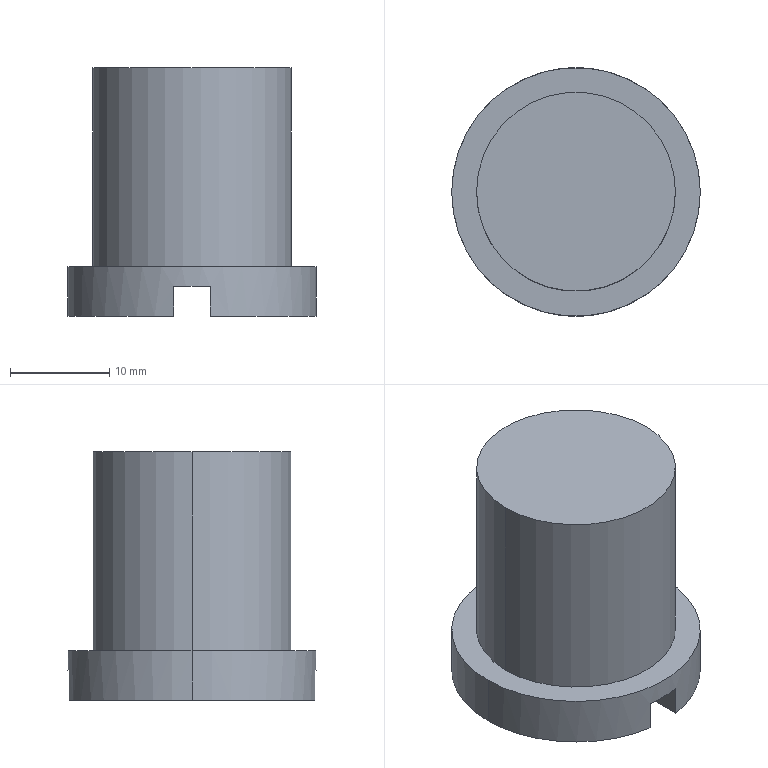Part | SolidWorks | features ICE 2, Extrusion 1 | 1 solid | 11 faces | box 25 x 25 x 25 mm | volume 8464 mm3 | plane 7 | cylinder 4 | commonest cylinder face diameters 20 x2 25 x2
STEP:
#1=CARTESIAN_POINT('',(10.,0.,25.));
#2=VERTEX_POINT('',#1);
#3=CARTESIAN_POINT('',(-10.,0.,25.));
#4=VERTEX_POINT('',#3);
#5=CARTESIAN_POINT('',(0.,0.,25.));
#6=DIRECTION('',(0.,0.,1.));
#7=DIRECTION('',(1.,0.,0.));
#8=AXIS2_PLACEMENT_3D('',#5,#6,#7);
#9=CIRCLE('',#8,10.);
#10=EDGE_CURVE('',#2,#4,#9,.T.);
#11=ORIENTED_EDGE('',*,*,#10,.F.);
#12=CARTESIAN_POINT('',(10.,0.,5.));
#13=VERTEX_POINT('',#12);
#14=CARTESIAN_POINT('',(10.,0.,25.));
#15=DIRECTION('',(0.,0.,-1.));
#16=VECTOR('',#15,1000.);
#17=LINE('',#14,#16);
#18=EDGE_CURVE('',#2,#13,#17,.T.);
#19=ORIENTED_EDGE('',*,*,#18,.T.);
#20=CARTESIAN_POINT('',(-10.,0.,5.));
#21=VERTEX_POINT('',#20);
#22=CARTESIAN_POINT('',(0.,0.,5.));
#23=DIRECTION('',(0.,0.,1.));
#24=DIRECTION('',(1.,0.,0.));
#25=AXIS2_PLACEMENT_3D('',#22,#23,#24);
#26=CIRCLE('',#25,10.);
#27=EDGE_CURVE('',#13,#21,#26,.T.);
#28=ORIENTED_EDGE('',*,*,#27,.T.);
#29=CARTESIAN_POINT('',(-10.,0.,25.));
#30=DIRECTION('',(0.,0.,-1.));
#31=VECTOR('',#30,1000.);
#32=LINE('',#29,#31);
#33=EDGE_CURVE('',#4,#21,#32,.T.);
#34=ORIENTED_EDGE('',*,*,#33,.F.);
#35=EDGE_LOOP('',(#11,#19,#28,#34));
#36=FACE_OUTER_BOUND('',#35,.T.);
#37=CARTESIAN_POINT('',(0.,0.,25.));
#38=DIRECTION('',(0.,0.,-1.));
#39=DIRECTION('',(-1.,0.,0.));
#40=AXIS2_PLACEMENT_3D('',#37,#38,#39);
#41=CYLINDRICAL_SURFACE('',#40,10.);
#42=ADVANCED_FACE('',(#36),#41,.T.);
#43=CARTESIAN_POINT('',(12.5,0.,5.));
#44=VERTEX_POINT('',#43);
#45=CARTESIAN_POINT('',(-12.5,0.,5.));
#46=VERTEX_POINT('',#45);
#47=CARTESIAN_POINT('',(0.,0.,5.));
#48=DIRECTION('',(0.,0.,1.));
#49=DIRECTION('',(1.,0.,0.));
#50=AXIS2_PLACEMENT_3D('',#47,#48,#49);
#51=CIRCLE('',#50,12.5);
#52=EDGE_CURVE('',#44,#46,#51,.T.);
#53=ORIENTED_EDGE('',*,*,#52,.F.);
#54=CARTESIAN_POINT('',(12.5,0.,0.));
#55=VERTEX_POINT('',#54);
#56=CARTESIAN_POINT('',(12.5,0.,5.));
#57=DIRECTION('',(0.,0.,-1.));
#58=VECTOR('',#57,1000.);
#59=LINE('',#56,#58);
#60=EDGE_CURVE('',#44,#55,#59,.T.);
#61=ORIENTED_EDGE('',*,*,#60,.T.);
#62=CARTESIAN_POINT('',(1.832,12.365,0.));
#63=VERTEX_POINT('',#62);
#64=CARTESIAN_POINT('',(0.,0.,0.));
#65=DIRECTION('',(0.,0.,1.));
#66=DIRECTION('',(1.,0.,0.));
#67=AXIS2_PLACEMENT_3D('',#64,#65,#66);
#68=CIRCLE('',#67,12.5);
#69=EDGE_CURVE('',#55,#63,#68,.T.);
#70=ORIENTED_EDGE('',*,*,#69,.T.);
#71=CARTESIAN_POINT('',(1.832,12.365,3.));
#72=VERTEX_POINT('',#71);
#73=CARTESIAN_POINT('',(1.832,12.365,3.));
#74=DIRECTION('',(0.,0.,-1.));
#75=VECTOR('',#74,1000.);
#76=LINE('',#73,#75);
#77=EDGE_CURVE('',#72,#63,#76,.T.);
#78=ORIENTED_EDGE('',*,*,#77,.F.);
#79=CARTESIAN_POINT('',(-1.832,12.365,3.));
#80=VERTEX_POINT('',#79);
#81=CARTESIAN_POINT('',(0.,0.,3.));
#82=DIRECTION('',(0.,0.,-1.));
#83=DIRECTION('',(-1.,0.,0.));
#84=AXIS2_PLACEMENT_3D('',#81,#82,#83);
#85=CIRCLE('',#84,12.5);
#86=EDGE_CURVE('',#80,#72,#85,.T.);
#87=ORIENTED_EDGE('',*,*,#86,.F.);
#88=CARTESIAN_POINT('',(-1.832,12.365,0.));
#89=VERTEX_POINT('',#88);
#90=CARTESIAN_POINT('',(-1.832,12.365,3.));
#91=DIRECTION('',(0.,0.,-1.));
#92=VECTOR('',#91,1000.);
#93=LINE('',#90,#92);
#94=EDGE_CURVE('',#80,#89,#93,.T.);
#95=ORIENTED_EDGE('',*,*,#94,.T.);
#96=CARTESIAN_POINT('',(-12.5,0.,0.));
#97=VERTEX_POINT('',#96);
#98=CARTESIAN_POINT('',(0.,0.,0.));
#99=DIRECTION('',(0.,0.,1.));
#100=DIRECTION('',(1.,0.,0.));
#101=AXIS2_PLACEMENT_3D('',#98,#99,#100);
#102=CIRCLE('',#101,12.5);
#103=EDGE_CURVE('',#89,#97,#102,.T.);
#104=ORIENTED_EDGE('',*,*,#103,.T.);
#105=CARTESIAN_POINT('',(-12.5,0.,5.));
#106=DIRECTION('',(0.,0.,-1.));
#107=VECTOR('',#106,1000.);
#108=LINE('',#105,#107);
#109=EDGE_CURVE('',#46,#97,#108,.T.);
#110=ORIENTED_EDGE('',*,*,#109,.F.);
#111=EDGE_LOOP('',(#53,#61,#70,#78,#87,#95,#104,#110));
#112=FACE_OUTER_BOUND('',#111,.T.);
#113=CARTESIAN_POINT('',(0.,0.,5.));
#114=DIRECTION('',(0.,0.,-1.));
#115=DIRECTION('',(-1.,0.,0.));
#116=AXIS2_PLACEMENT_3D('',#113,#114,#115);
#117=CYLINDRICAL_SURFACE('',#116,12.5);
#118=ADVANCED_FACE('',(#112),#117,.T.);
#119=ORIENTED_EDGE('',*,*,#103,.F.);
#120=CARTESIAN_POINT('',(-1.832,-12.365,0.));
#121=VERTEX_POINT('',#120);
#122=CARTESIAN_POINT('',(-1.832,12.365,0.));
#123=DIRECTION('',(0.,1.,0.));
#124=VECTOR('',#123,1000.);
#125=LINE('',#122,#124);
#126=EDGE_CURVE('',#121,#89,#125,.T.);
#127=ORIENTED_EDGE('',*,*,#126,.F.);
#128=CARTESIAN_POINT('',(0.,0.,0.));
#129=DIRECTION('',(0.,0.,1.));
#130=DIRECTION('',(1.,0.,0.));
#131=AXIS2_PLACEMENT_3D('',#128,#129,#130);
#132=CIRCLE('',#131,12.5);
#133=EDGE_CURVE('',#97,#121,#132,.T.);
#134=ORIENTED_EDGE('',*,*,#133,.F.);
#135=EDGE_LOOP('',(#119,#127,#134));
#136=FACE_OUTER_BOUND('',#135,.T.);
#137=CARTESIAN_POINT('',(0.,0.,0.));
#138=DIRECTION('',(0.,0.,1.));
#139=DIRECTION('',(1.,0.,0.));
#140=AXIS2_PLACEMENT_3D('',#137,#138,#139);
#141=PLANE('',#140);
#142=ADVANCED_FACE('',(#136),#141,.F.);
#143=ORIENTED_EDGE('',*,*,#60,.F.);
#144=CARTESIAN_POINT('',(0.,0.,5.));
#145=DIRECTION('',(0.,0.,1.));
#146=DIRECTION('',(1.,0.,0.));
#147=AXIS2_PLACEMENT_3D('',#144,#145,#146);
#148=CIRCLE('',#147,12.5);
#149=EDGE_CURVE('',#46,#44,#148,.T.);
#150=ORIENTED_EDGE('',*,*,#149,.F.);
#151=ORIENTED_EDGE('',*,*,#109,.T.);
#152=ORIENTED_EDGE('',*,*,#133,.T.);
#153=CARTESIAN_POINT('',(-1.832,-12.365,3.));
#154=VERTEX_POINT('',#153);
#155=CARTESIAN_POINT('',(-1.832,-12.365,3.));
#156=DIRECTION('',(0.,0.,-1.));
#157=VECTOR('',#156,1000.);
#158=LINE('',#155,#157);
#159=EDGE_CURVE('',#154,#121,#158,.T.);
#160=ORIENTED_EDGE('',*,*,#159,.F.);
#161=CARTESIAN_POINT('',(1.832,-12.365,3.));
#162=VERTEX_POINT('',#161);
#163=CARTESIAN_POINT('',(0.,0.,3.));
#164=DIRECTION('',(0.,0.,-1.));
#165=DIRECTION('',(-1.,0.,0.));
#166=AXIS2_PLACEMENT_3D('',#163,#164,#165);
#167=CIRCLE('',#166,12.5);
#168=EDGE_CURVE('',#162,#154,#167,.T.);
#169=ORIENTED_EDGE('',*,*,#168,.F.);
#170=CARTESIAN_POINT('',(1.832,-12.365,0.));
#171=VERTEX_POINT('',#170);
#172=CARTESIAN_POINT('',(1.832,-12.365,3.));
#173=DIRECTION('',(0.,0.,-1.));
#174=VECTOR('',#173,1000.);
#175=LINE('',#172,#174);
#176=EDGE_CURVE('',#162,#171,#175,.T.);
#177=ORIENTED_EDGE('',*,*,#176,.T.);
#178=CARTESIAN_POINT('',(0.,0.,0.));
#179=DIRECTION('',(0.,0.,1.));
#180=DIRECTION('',(1.,0.,0.));
#181=AXIS2_PLACEMENT_3D('',#178,#179,#180);
#182=CIRCLE('',#181,12.5);
#183=EDGE_CURVE('',#171,#55,#182,.T.);
#184=ORIENTED_EDGE('',*,*,#183,.T.);
#185=EDGE_LOOP('',(#143,#150,#151,#152,#160,#169,#177,#184));
#186=FACE_OUTER_BOUND('',#185,.T.);
#187=CARTESIAN_POINT('',(0.,0.,5.));
#188=DIRECTION('',(0.,0.,-1.));
#189=DIRECTION('',(-1.,0.,0.));
#190=AXIS2_PLACEMENT_3D('',#187,#188,#189);
#191=CYLINDRICAL_SURFACE('',#190,12.5);
#192=ADVANCED_FACE('',(#186),#191,.T.);
#193=CARTESIAN_POINT('',(0.,0.,5.));
#194=DIRECTION('',(0.,0.,1.));
#195=DIRECTION('',(1.,0.,0.));
#196=AXIS2_PLACEMENT_3D('',#193,#194,#195);
#197=CIRCLE('',#196,10.);
#198=EDGE_CURVE('',#21,#13,#197,.T.);
#199=ORIENTED_EDGE('',*,*,#198,.F.);
#200=ORIENTED_EDGE('',*,*,#27,.F.);
#201=EDGE_LOOP('',(#199,#200));
#202=FACE_BOUND('',#201,.T.);
#203=ORIENTED_EDGE('',*,*,#149,.T.);
#204=ORIENTED_EDGE('',*,*,#52,.T.);
#205=EDGE_LOOP('',(#203,#204));
#206=FACE_OUTER_BOUND('',#205,.T.);
#207=CARTESIAN_POINT('',(0.,0.,5.));
#208=DIRECTION('',(0.,0.,1.));
#209=DIRECTION('',(1.,0.,0.));
#210=AXIS2_PLACEMENT_3D('',#207,#208,#209);
#211=PLANE('',#210);
#212=ADVANCED_FACE('',(#202,#206),#211,.T.);
#213=ORIENTED_EDGE('',*,*,#183,.F.);
#214=CARTESIAN_POINT('',(1.832,12.365,0.));
#215=DIRECTION('',(0.,-1.,0.));
#216=VECTOR('',#215,1000.);
#217=LINE('',#214,#216);
#218=EDGE_CURVE('',#63,#171,#217,.T.);
#219=ORIENTED_EDGE('',*,*,#218,.F.);
#220=ORIENTED_EDGE('',*,*,#69,.F.);
#221=EDGE_LOOP('',(#213,#219,#220));
#222=FACE_OUTER_BOUND('',#221,.T.);
#223=CARTESIAN_POINT('',(0.,0.,0.));
#224=DIRECTION('',(0.,0.,1.));
#225=DIRECTION('',(1.,0.,0.));
#226=AXIS2_PLACEMENT_3D('',#223,#224,#225);
#227=PLANE('',#226);
#228=ADVANCED_FACE('',(#222),#227,.F.);
#229=ORIENTED_EDGE('',*,*,#18,.F.);
#230=CARTESIAN_POINT('',(0.,0.,25.));
#231=DIRECTION('',(0.,0.,1.));
#232=DIRECTION('',(1.,0.,0.));
#233=AXIS2_PLACEMENT_3D('',#230,#231,#232);
#234=CIRCLE('',#233,10.);
#235=EDGE_CURVE('',#4,#2,#234,.T.);
#236=ORIENTED_EDGE('',*,*,#235,.F.);
#237=ORIENTED_EDGE('',*,*,#33,.T.);
#238=ORIENTED_EDGE('',*,*,#198,.T.);
#239=EDGE_LOOP('',(#229,#236,#237,#238));
#240=FACE_OUTER_BOUND('',#239,.T.);
#241=CARTESIAN_POINT('',(0.,0.,25.));
#242=DIRECTION('',(0.,0.,-1.));
#243=DIRECTION('',(-1.,0.,0.));
#244=AXIS2_PLACEMENT_3D('',#241,#242,#243);
#245=CYLINDRICAL_SURFACE('',#244,10.);
#246=ADVANCED_FACE('',(#240),#245,.T.);
#247=ORIENTED_EDGE('',*,*,#235,.T.);
#248=ORIENTED_EDGE('',*,*,#10,.T.);
#249=EDGE_LOOP('',(#247,#248));
#250=FACE_OUTER_BOUND('',#249,.T.);
#251=CARTESIAN_POINT('',(0.,0.,25.));
#252=DIRECTION('',(0.,0.,1.));
#253=DIRECTION('',(1.,0.,0.));
#254=AXIS2_PLACEMENT_3D('',#251,#252,#253);
#255=PLANE('',#254);
#256=ADVANCED_FACE('',(#250),#255,.T.);
#257=ORIENTED_EDGE('',*,*,#126,.T.);
#258=ORIENTED_EDGE('',*,*,#94,.F.);
#259=CARTESIAN_POINT('',(-1.832,12.365,3.));
#260=DIRECTION('',(0.,1.,0.));
#261=VECTOR('',#260,1000.);
#262=LINE('',#259,#261);
#263=EDGE_CURVE('',#154,#80,#262,.T.);
#264=ORIENTED_EDGE('',*,*,#263,.F.);
#265=ORIENTED_EDGE('',*,*,#159,.T.);
#266=EDGE_LOOP('',(#257,#258,#264,#265));
#267=FACE_OUTER_BOUND('',#266,.T.);
#268=CARTESIAN_POINT('',(-1.832,12.365,3.));
#269=DIRECTION('',(-1.,0.,0.));
#270=DIRECTION('',(0.,-1.,0.));
#271=AXIS2_PLACEMENT_3D('',#268,#269,#270);
#272=PLANE('',#271);
#273=ADVANCED_FACE('',(#267),#272,.F.);
#274=ORIENTED_EDGE('',*,*,#218,.T.);
#275=ORIENTED_EDGE('',*,*,#176,.F.);
#276=CARTESIAN_POINT('',(1.832,12.365,3.));
#277=DIRECTION('',(0.,-1.,0.));
#278=VECTOR('',#277,1000.);
#279=LINE('',#276,#278);
#280=EDGE_CURVE('',#72,#162,#279,.T.);
#281=ORIENTED_EDGE('',*,*,#280,.F.);
#282=ORIENTED_EDGE('',*,*,#77,.T.);
#283=EDGE_LOOP('',(#274,#275,#281,#282));
#284=FACE_OUTER_BOUND('',#283,.T.);
#285=CARTESIAN_POINT('',(1.832,12.365,3.));
#286=DIRECTION('',(1.,0.,0.));
#287=DIRECTION('',(0.,1.,0.));
#288=AXIS2_PLACEMENT_3D('',#285,#286,#287);
#289=PLANE('',#288);
#290=ADVANCED_FACE('',(#284),#289,.F.);
#291=ORIENTED_EDGE('',*,*,#86,.T.);
#292=ORIENTED_EDGE('',*,*,#280,.T.);
#293=ORIENTED_EDGE('',*,*,#168,.T.);
#294=ORIENTED_EDGE('',*,*,#263,.T.);
#295=EDGE_LOOP('',(#291,#292,#293,#294));
#296=FACE_OUTER_BOUND('',#295,.T.);
#297=CARTESIAN_POINT('',(0.,0.,3.));
#298=DIRECTION('',(0.,0.,-1.));
#299=DIRECTION('',(-1.,0.,0.));
#300=AXIS2_PLACEMENT_3D('',#297,#298,#299);
#301=PLANE('',#300);
#302=ADVANCED_FACE('',(#296),#301,.T.);
#303=CLOSED_SHELL('',(#42,#118,#142,#192,#212,#228,#246,#256,#273,#290,#302));
#304=MANIFOLD_SOLID_BREP('',#303);
#305=CARTESIAN_POINT('',(0.,0.,0.));
#306=DIRECTION('',(0.,0.,1.));
#307=DIRECTION('',(1.,0.,0.));
#308=AXIS2_PLACEMENT_3D('',#305,#306,#307);
#309=(LENGTH_UNIT()NAMED_UNIT(*)SI_UNIT(.MILLI.,.METRE.));
#310=UNCERTAINTY_MEASURE_WITH_UNIT(LENGTH_MEASURE(0.00001),#309,'','');
#311=(NAMED_UNIT(*)PLANE_ANGLE_UNIT()SI_UNIT($,.RADIAN.));
#312=(NAMED_UNIT(*)SI_UNIT($,.STERADIAN.)SOLID_ANGLE_UNIT());
#313=(GEOMETRIC_REPRESENTATION_CONTEXT(3)GLOBAL_UNCERTAINTY_ASSIGNED_CONTEXT((#310))GLOBAL_UNIT_ASSIGNED_CONTEXT((#309,#311,#312))REPRESENTATION_CONTEXT('',''));
#314=ADVANCED_BREP_SHAPE_REPRESENTATION('',(#304,#308),#313);